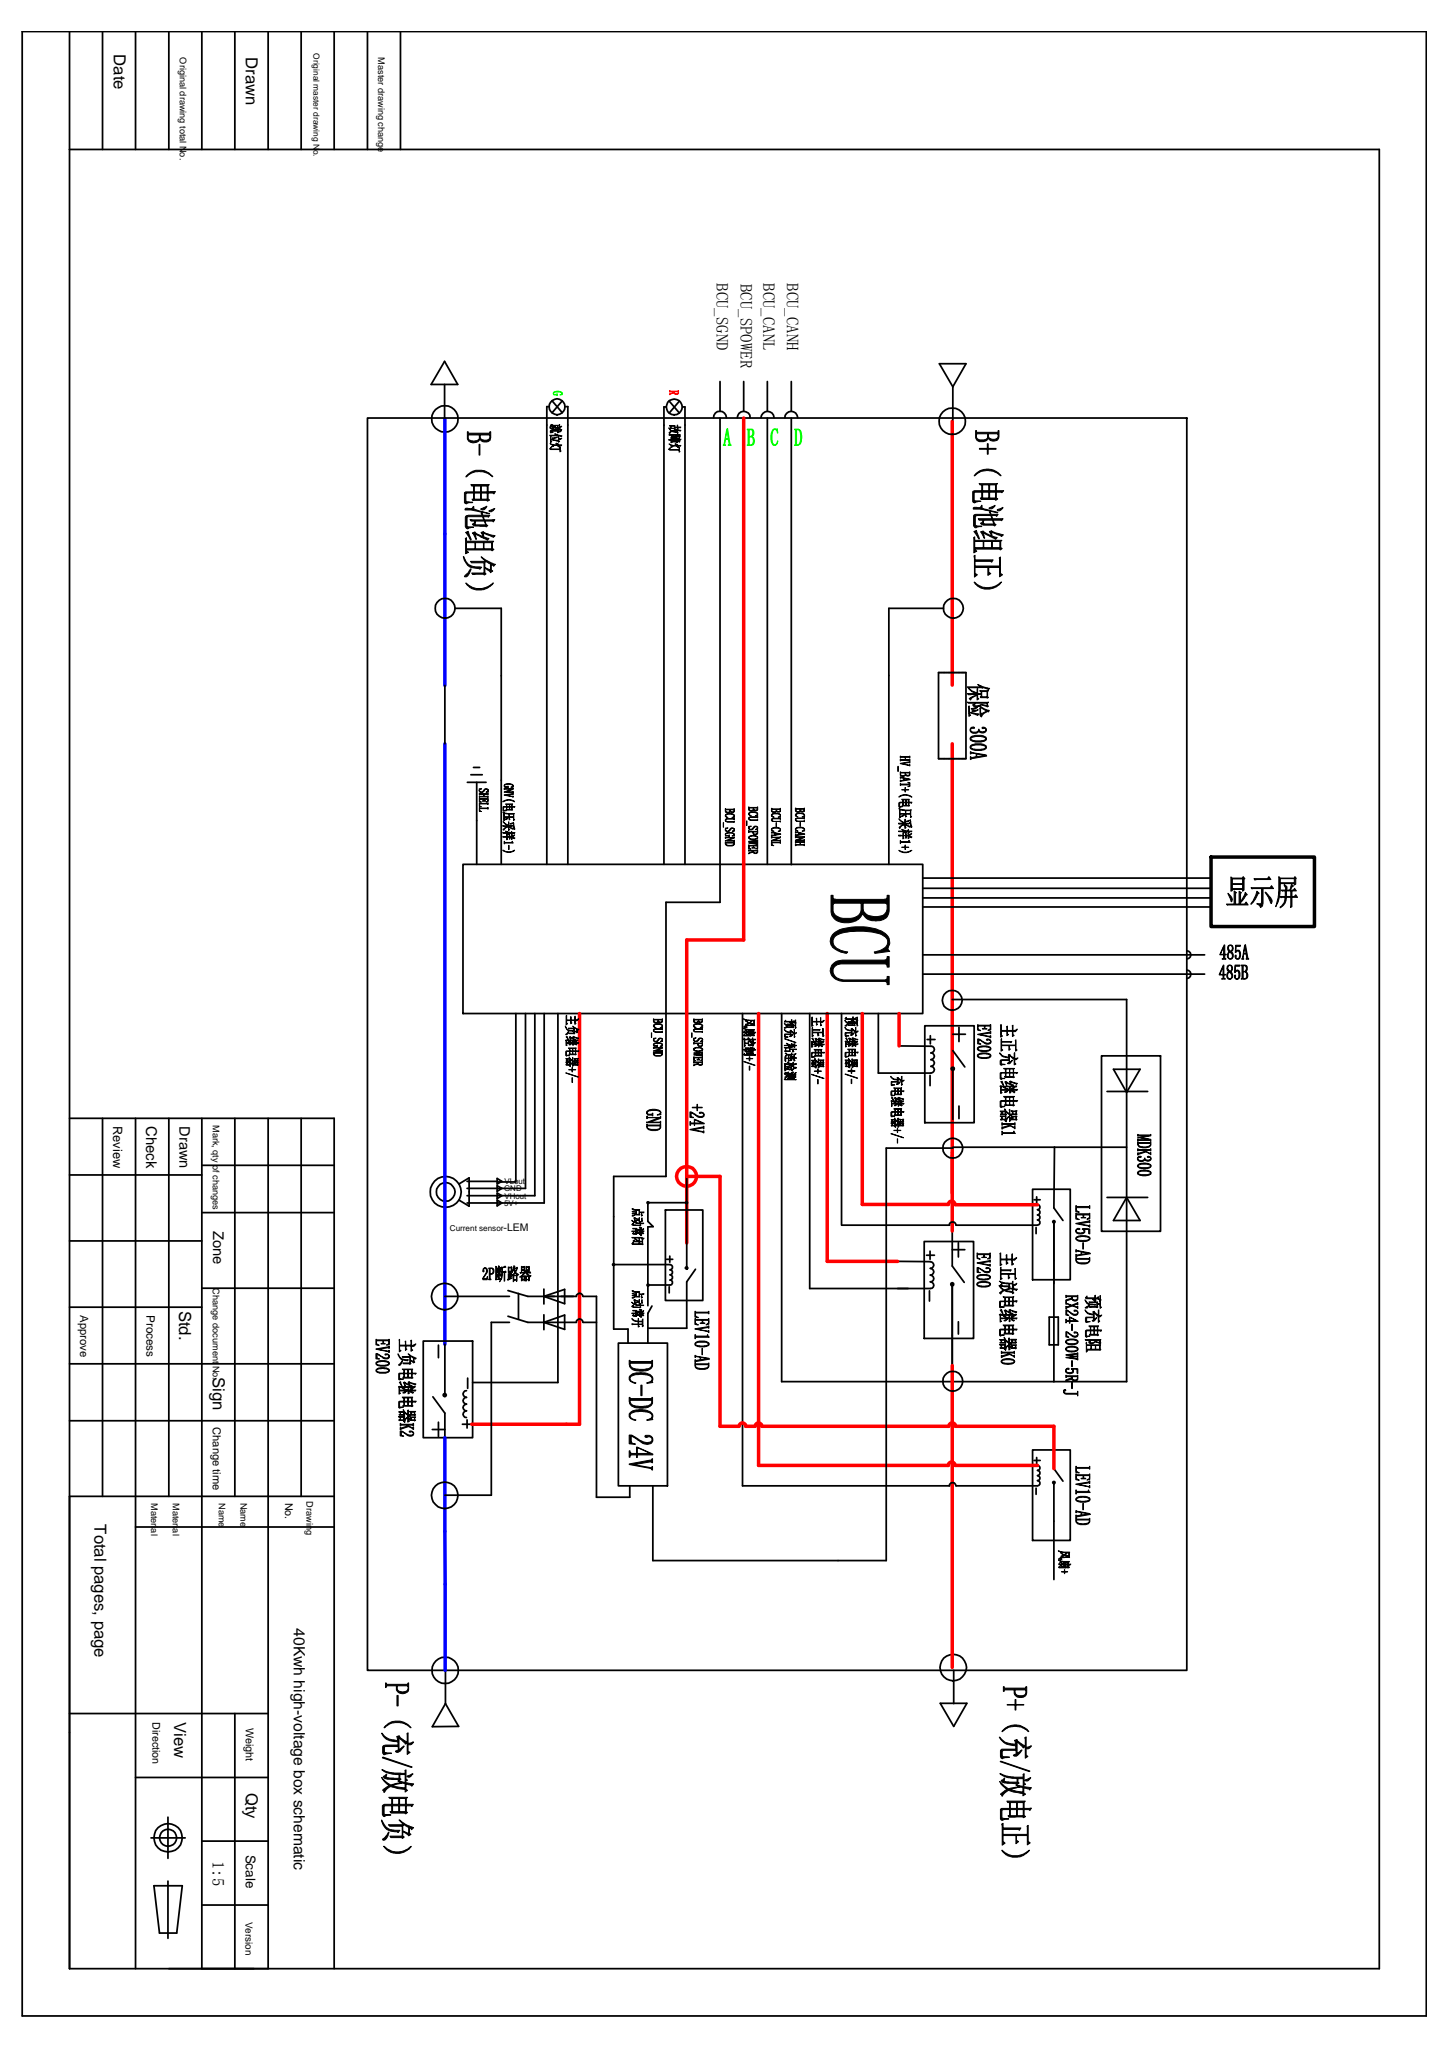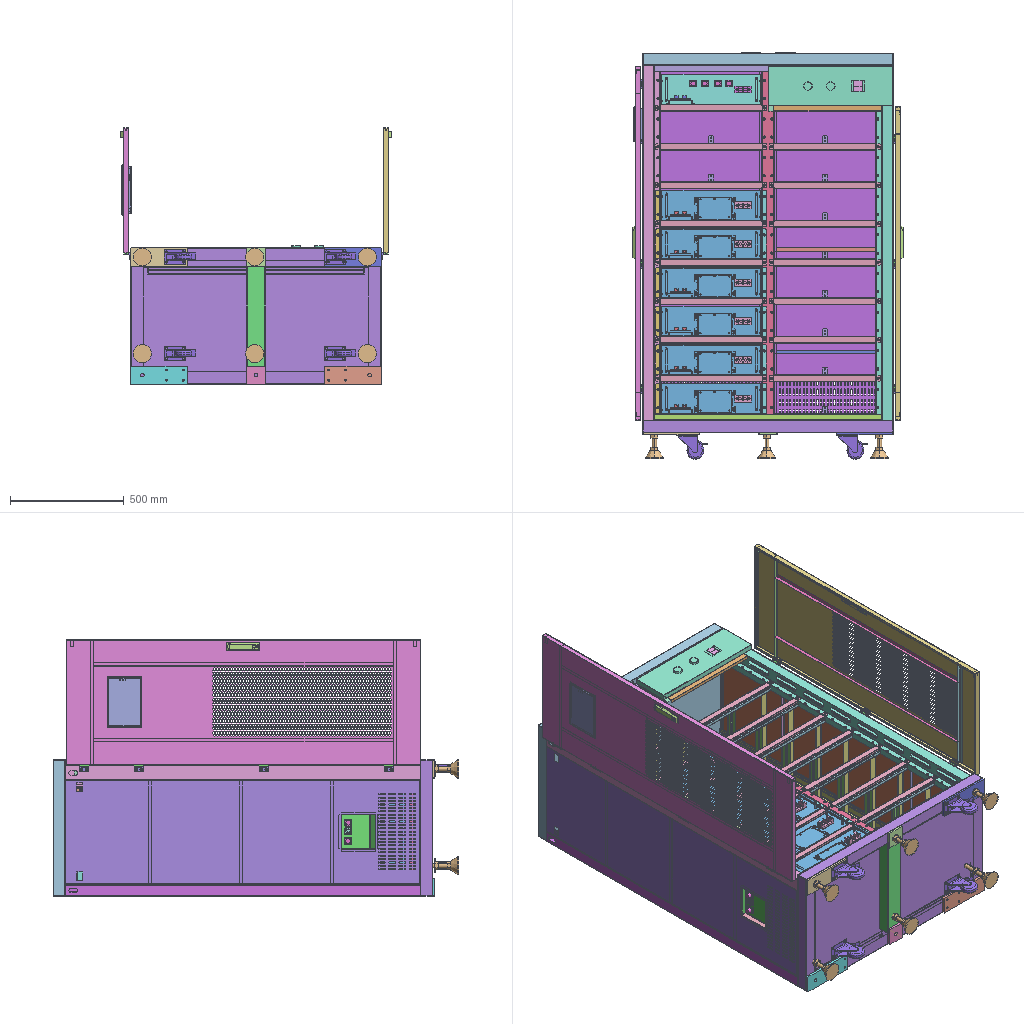Assembly | SolidWorks | 125 different items | 547 placed | box 1190 x 1786 x 1129 mm
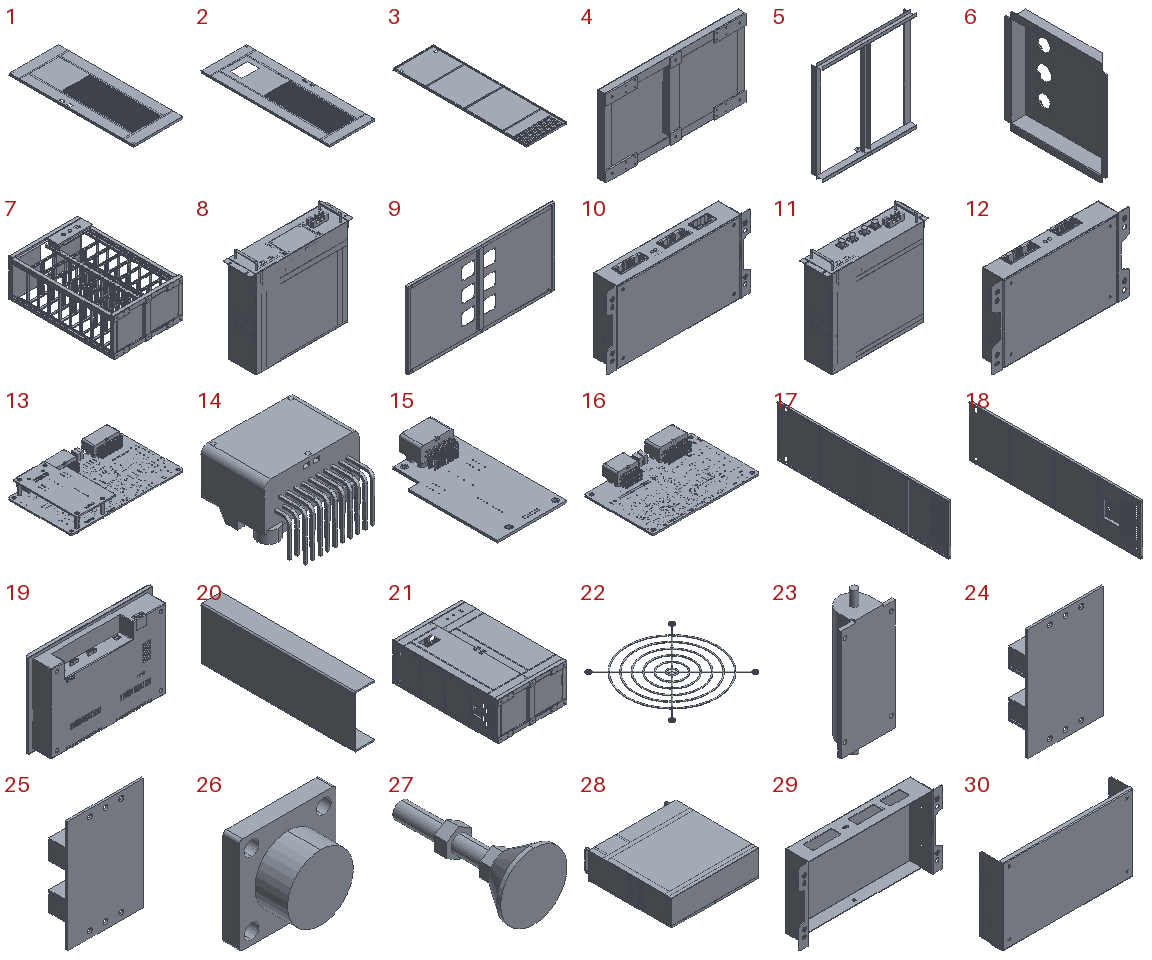Parts list (item | name | quantity | parent item | size | volume | features):
1 | (subassembly) | x1 | - | - | 1001235 mm3 | features MirrorCompFeat 1, ReferencePattern 1
2 | (subassembly) | x1 | - | - | 1107587 mm3 | features MirrorCompFeat 1, ReferencePattern 1
3 | (subassembly) | x2 | - | 473 x 1568 x 20 mm | 883759 mm3 | features CompositeCurve 2
4 | (subassembly) | x1 | in 7 | 1100 x 63 x 600.001 mm | 2743089 mm3 | -
5 | (subassembly) | x17 | in 7 | 453 x 63.5 x 481.5 mm | 236917 mm3 | -
6 | (subassembly) | x1 | in 18 | 29 x 171 x 172 mm | 45900 mm3 | -
7 | (subassembly) | x1 | - | - | 11157281 mm3 | features ReferencePattern 16, LocalLPattern 1
8 | (subassembly) | x6 | - | - | 10284410 mm3 | features ReferencePattern 16, CompositeCurve 5, LocalLPattern 2, MirrorCompFeat 1
9 | (subassembly) | x1 | - | 1035 x 20 x 535 mm | 656761 mm3 | -
10 | (subassembly) | x1 | in 11 | - | 121145 mm3 | -
11 | (subassembly) | x1 | - | - | 2990736 mm3 | features CompositeCurve 17, LocalLPattern 3, ReferencePattern 3
12 | (subassembly) | x6 | in 8 | 177.9 x 27.2 x 101.3 mm | 74977 mm3 | -
13 | (subassembly) | x1 | in 10 | - | 62246 mm3 | -
14 | (subassembly) | x1 | in 15 | 27.9 x 26.52 x 19.2 mm | 3570 mm3 | -
15 | (subassembly) | x1 | in 13 | 60 x 105.587 x 19.2 mm | 14940 mm3 | -
16 | (subassembly) | x6 | in 12 | 137.5 x 94.8 x 23.5 mm | 33178 mm3 | -
17 | (subassembly) | x1 | - | 20 x 1568 x 458 mm | 1656594 mm3 | features CompositeCurve 2
18 | (subassembly) | x1 | - | 30 x 1568 x 458 mm | 871583 mm3 | features CompositeCurve 3, LocalLPattern 1, ReferencePattern 1
19 | - | x1 | - | 227 x 40.02 x 153 mm | 206698 mm3 | features BaseBody 27
20 | - | x1 | in 7 | 23.5 x 176 x 60 mm | 27263 mm3 | features SplitBody 1
21 | - | x0 | - | - | 13322104 mm3 | features ICE 63, FlatPattern 34, SMBaseFlange 34, SheetMetal 34, LPattern 21, MirrorSolid 19, EdgeFlange 14, BossThin 9, MirrorPattern 6, SMMiteredFlange 6, Chamfer 2, CornerTrim 1, Split 1
22 | - | x6 | - | 89 x 89 x 1 mm | 913.094 mm3 | features Fillet 4, ICE 3, Extrusion 1, Revolution 1
23 | - | x1 | in 11 | 48 x 25.9 x 126 mm | 68546 mm3 | features ICE 7, Extrusion 1
24 | - | x6 | in 8 | 60.4 x 15.3 x 89.7 mm | 16280 mm3 | features ICE 4, Extrusion 1
25 | - | x1 | in 11 | 60.4 x 15.3 x 89.7 mm | 16562 mm3 | features ICE 3, Extrusion 1
26 | - | x1 | - | 29.5 x 17 x 29.5 mm | 7218 mm3 | features ICE 5, Extrusion 1, Fillet 1
27 | - | x6 | - | 80 x 160 x 80 mm | 165736 mm3 | features ICE 4, Extrusion 1
28 | - | x1 | in 11 | 437 x 449.5 x 132 mm | 767937 mm3 | features ICE 25, BossThin 16, LPattern 10, EdgeFlange 7, SMBaseFlange 7, FlatPattern 6, SheetMetal 6, MirrorPattern 4, CornerTrim 2, MirrorSolid 1, Split 1, Sweep 1
29 | - | x1 | in 10 | 216.4 x 35.2 x 109.5 mm | 30574 mm3 | features BaseBody 5
30 | - | x1 | in 10 | 185.4 x 34 x 108 mm | 28122 mm3 | features BaseBody 6
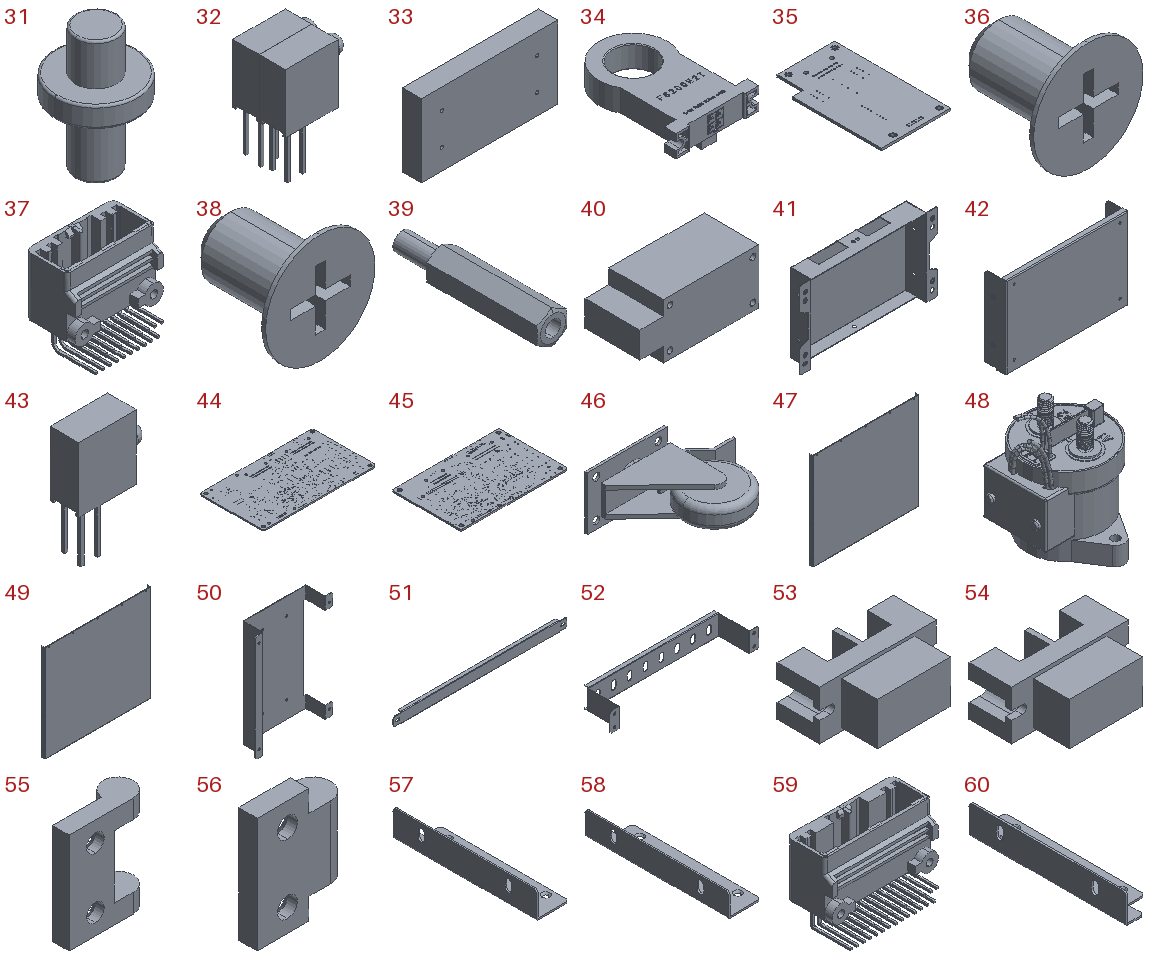31 | - | x8 | in 3, 17, 18 | 8 x 8 x 12 mm | 225.557 mm3 | features Fillet 2, ICE 2, Extrusion 1
32 | - | x1 | in 13 | 11.4 x 8.95 x 17.5 mm | 805.198 mm3 | features BaseBody 2
33 | - | x1 | in 11 | 215 x 30 x 115 mm | 739394 mm3 | features Extrusion 1, ICE 1
34 | - | x1 | in 11 | 56 x 80 x 24.3 mm | 37324 mm3 | features BaseBody 5
35 | - | x1 | in 15 | 60 x 100 x 2.001 mm | 11370 mm3 | features BaseBody 1
36 | - | x30 | in 12 | 5.5 x 5 x 5.5 mm | 40.626 mm3 | features BaseBody 1
37 | - | x6 | in 16 | 27.9 x 19.2 x 26.52 mm | 3570 mm3 | features BaseBody 1
38 | - | x5 | in 10 | 5.5 x 5 x 5.5 mm | 40.626 mm3 | features BaseBody 1
39 | - | x4 | in 13 | 4.7 x 24 x 5.427 mm | 364.722 mm3 | features BaseBody 1
40 | - | x1 | in 11 | 115 x 53 x 53 mm | 283866 mm3 | features ICE 2, Extrusion 1
41 | - | x6 | in 12 | 177.9 x 27.2 x 100 mm | 21775 mm3 | features BaseBody 5, ICE 2
42 | - | x6 | in 12 | 146.9 x 26 x 98.5 mm | 19821 mm3 | features BaseBody 6
43 | - | x12 | in 16 | 11.4 x 4.45 x 17.5 mm | 402.599 mm3 | features BaseBody 1
44 | - | x1 | in 13 | 177 x 100 x 2 mm | 34913 mm3 | features BaseBody 1
45 | - | x6 | in 16 | 137.5 x 89 x 2 mm | 24002 mm3 | features BaseBody 1
46 | - | x4 | - | 138.347 x 107 x 64 mm | 180748 mm3 | features ICE 7, BossThin 1, Extrusion 1, Fillet 1, MirrorPattern 1
47 | - | x6 | in 8 | 437.001 x 12.7 x 399 mm | 225419 mm3 | features ICE 3, LPattern 3, EdgeFlange 1, FlatPattern 1, SMBaseFlange 1, SheetMetal 1
48 | - | x3 | in 11 | - | - | features BaseBody 14, RefSurface 2
49 | - | x1 | in 11 | 437.001 x 12.7 x 399 mm | 225419 mm3 | features ICE 3, LPattern 3, EdgeFlange 1, FlatPattern 1, SMBaseFlange 1, SheetMetal 1
50 | - | x1 | in 11 | 160 x 41 x 220 mm | 42307 mm3 | features ICE 3, CornerTrim 1, FlatPattern 1, SMBaseFlange 1, SheetMetal 1
51 | - | x17 | - | 490 x 9.5 x 29 mm | 30933 mm3 | features CornerTrim 2, ICE 2, EdgeFlange 1, FlatPattern 1, SMBaseFlange 1, SheetMetal 1
52 | - | x12 | in 8 | 385 x 91.2 x 52.6 mm | 39000 mm3 | features CornerTrim 2, ICE 2, EdgeFlange 1, FlatPattern 1, LPattern 1, MirrorPattern 1, SMBaseFlange 1, SheetMetal 1
53 | - | x7 | in 8, 11 | 71 x 48 x 30 mm | 59444 mm3 | features ICE 5, LPattern 2, Extrusion 1
54 | - | x1 | in 11 | 71 x 48 x 30 mm | 59444 mm3 | features ICE 5, LPattern 2, Extrusion 1
55 | - | x7 | - | 31.5 x 12 x 40 mm | 5884 mm3 | features ICE 3, Chamfer 1, Extrusion 1
56 | - | x7 | - | 31.5 x 12 x 40 mm | 7190 mm3 | features ICE 3, Chamfer 1, Extrusion 1
57 | - | x6 | in 8 | 30 x 132 x 24.5 mm | 9772 mm3 | features ICE 3, CornerTrim 2, Chamfer 1, EdgeFlange 1, FlatPattern 1, SMBaseFlange 1, SheetMetal 1
58 | - | x1 | in 11 | 30 x 132 x 21.5 mm | 9178 mm3 | features ICE 3, CornerTrim 2, Chamfer 1, EdgeFlange 1, FlatPattern 1, SMBaseFlange 1, SheetMetal 1
59 | - | x6 | in 16 | 36.7 x 19.2 x 26.52 mm | 4801 mm3 | features BaseBody 1
60 | - | x6 | in 8 | 30 x 132 x 24.5 mm | 9772 mm3 | features ICE 3, CornerTrim 2, Chamfer 1, EdgeFlange 1, FlatPattern 1, SMBaseFlange 1, SheetMetal 1
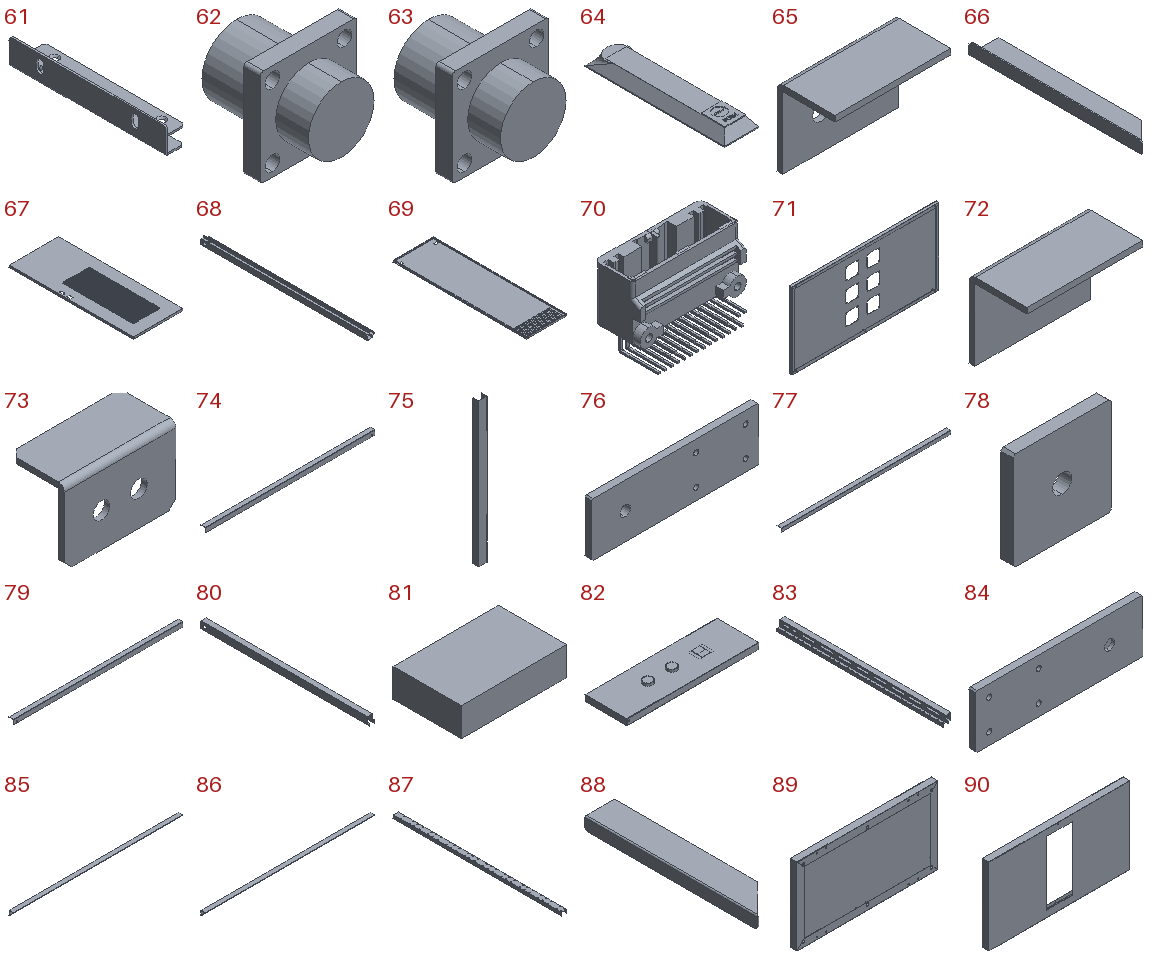61 | - | x1 | in 11 | 30 x 132 x 21.5 mm | 9178 mm3 | features ICE 3, CornerTrim 2, Chamfer 1, EdgeFlange 1, FlatPattern 1, SMBaseFlange 1, SheetMetal 1
62 | - | x2 | in 18 | 29.5 x 32 x 29.5 mm | 13059 mm3 | features ICE 3, Extrusion 1, Fillet 1
63 | - | x7 | in 11 | 29.5 x 32 x 29.5 mm | 13059 mm3 | features ICE 3, Extrusion 1, Fillet 1
64 | - | x2 | - | 36 x 147 x 22 mm | 47748 mm3 | features ICE 7, Blend 1
65 | - | x1 | in 1 | 30 x 15 x 20 mm | 1467 mm3 | features SplitBody 1
66 | - | x2 | in 6 | 26 x 152.414 x 11 mm | 5106 mm3 | features Chamfer 1, SplitBody 1
67 | - | x1 | in 1 | - | 901545 mm3 | features APattern 1, ICE 1, SplitBody 1
68 | - | x1 | in 7 | 75 x 1562 x 70 mm | 454767 mm3 | features SplitBody 1
69 | - | x2 | in 3 | 473 x 1560 x 20 mm | 829157 mm3 | features LPattern 2, ICE 1, SplitBody 1
70 | - | x1 | in 13 | 36.7 x 19.2 x 26.52 mm | 4801 mm3 | features BaseBody 1
71 | - | x1 | in 9 | 1035 x 20 x 535 mm | 624346 mm3 | features SplitBody 1
72 | - | x1 | in 2 | 30 x 15 x 20 mm | 1467 mm3 | features SplitBody 1
73 | - | x1 | in 1 | 30 x 15 x 20 mm | 1431 mm3 | features Chamfer 1, ICE 1, SplitBody 1
74 | - | x1 | in 2 | 547.1 x 15 x 15 mm | 15709 mm3 | features SplitBody 1
75 | - | x1 | in 9 | 30 x 19 x 495 mm | 32415 mm3 | features SplitBody 1
76 | - | x1 | in 4 | 250 x 10 x 80 mm | 196266 mm3 | features ICE 1, SplitBody 1
77 | - | x1 | in 7 | 1000 x 26.5 x 20 mm | 66953 mm3 | features SplitBody 1
78 | - | x1 | in 4 | 80 x 10 x 80 mm | 62033 mm3 | features SplitBody 1
79 | - | x1 | in 1 | 547.1 x 15 x 15 mm | 15709 mm3 | features SplitBody 1
80 | - | x1 | in 7 | 75 x 1562 x 90 mm | 569979 mm3 | features SplitBody 1
81 | - | x96 | in 8 | 148.9 x 100.6 x 40.2 mm | 574008 mm3 | features Extrusion 1, ICE 1
82 | - | x1 | in 7 | 548.5 x 174 x 73 mm | 187457 mm3 | features ICE 5, EdgeFlange 2, FlatPattern 2, SheetMetal 2, BossThin 1, CornerTrim 1, MirrorSolid 1, SMBaseFlange 1, SplitBody 1
83 | - | x1 | in 7 | 75 x 1562 x 90 mm | 568326 mm3 | features SplitBody 1
84 | - | x1 | in 4 | 250 x 10 x 80 mm | 198093 mm3 | features SplitBody 1
85 | - | x1 | in 2 | 547.1 x 15 x 15 mm | 15709 mm3 | features SplitBody 1
86 | - | x1 | in 1 | 547.1 x 15 x 15 mm | 15693 mm3 | features ICE 1, SplitBody 1
87 | - | x1 | in 7 | 50 x 1562 x 30 mm | 258598 mm3 | features SplitBody 1
88 | - | x1 | in 6 | 26 x 152.414 x 11 mm | 5106 mm3 | features Chamfer 1, SplitBody 1
89 | - | x1 | in 4 | 1100 x 53 x 600.001 mm | 1504531 mm3 | features SplitBody 1
90 | - | x1 | in 7 | 1100 x 53 x 600.001 mm | 1427839 mm3 | features SplitBody 1
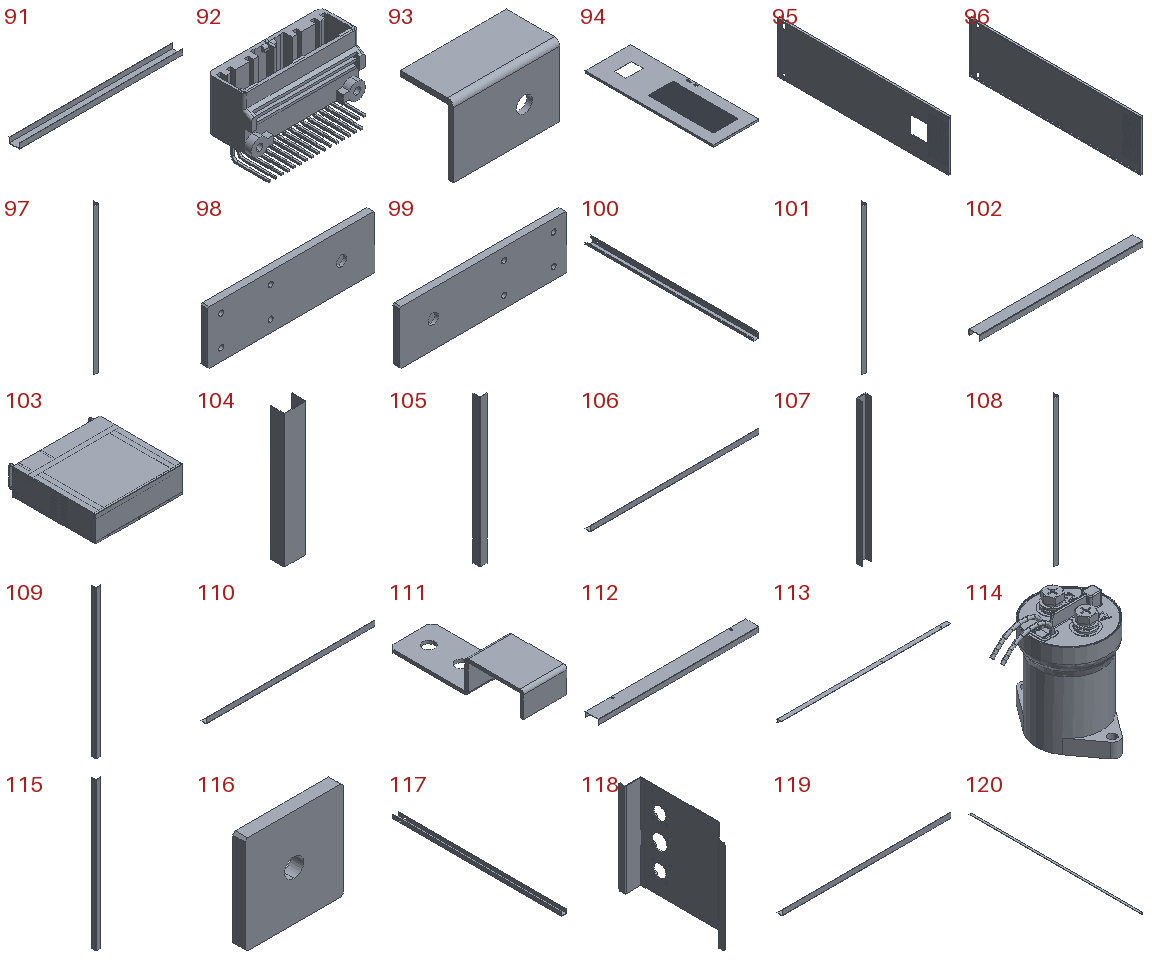91 | - | x17 | in 5 | 450 x 30 x 15 mm | 37982 mm3 | features SplitBody 1
92 | - | x1 | in 13 | 41.1 x 19.2 x 26.52 mm | 5328 mm3 | features BaseBody 1
93 | - | x1 | in 2 | 30 x 15 x 20 mm | 1467 mm3 | features SplitBody 1
94 | - | x1 | in 2 | - | 997556 mm3 | features APattern 1, ICE 1, SplitBody 1
95 | - | x1 | in 18 | 20 x 1560 x 458 mm | 785912 mm3 | features SplitBody 1
96 | - | x2 | in 17 | 20 x 1560 x 458 mm | 808412 mm3 | features SplitBody 1
97 | - | x1 | in 17 | 15 x 15 x 456 mm | 13107 mm3 | features SplitBody 1
98 | - | x1 | in 4 | 250 x 10 x 80 mm | 198093 mm3 | features SplitBody 1
99 | - | x1 | in 4 | 250 x 10 x 80 mm | 198093 mm3 | features SplitBody 1
100 | - | x1 | in 7 | 75 x 1562 x 70 mm | 454767 mm3 | features SplitBody 1
101 | - | x1 | in 17 | 15 x 15 x 456 mm | 13107 mm3 | features SplitBody 1
102 | - | x17 | in 5 | 450 x 30 x 15 mm | 37982 mm3 | features SplitBody 1
103 | - | x6 | in 8 | 437 x 449.5 x 132 mm | 626623 mm3 | features ICE 15, LPattern 7, SMBaseFlange 7, EdgeFlange 6, FlatPattern 6, SheetMetal 6, MirrorPattern 4, BossThin 3, CornerTrim 2, MirrorSolid 1, Split 1, Sweep 1
104 | - | x2 | in 4 | 80 x 51.5 x 487 mm | 130957 mm3 | features SplitBody 1
105 | - | x17 | in 5 | 21.5 x 21.5 x 450 mm | 27766 mm3 | features SplitBody 1
106 | - | x4 | in 3 | 471 x 15 x 15 mm | 13538 mm3 | features SplitBody 1
107 | - | x34 | in 5 | 30 x 20 x 450 mm | 44732 mm3 | features SplitBody 1
108 | - | x1 | in 17 | 15 x 15 x 456 mm | 13107 mm3 | features SplitBody 1
109 | - | x1 | in 18 | 15 x 15 x 456 mm | 13107 mm3 | features SplitBody 1
110 | - | x2 | in 3 | 471 x 15 x 15 mm | 13538 mm3 | features SplitBody 1
111 | - | x17 | in 5 | 20 x 62 x 15 mm | 2455 mm3 | features SplitBody 1
112 | - | x1 | in 7 | 475 x 40 x 15 mm | 32008 mm3 | features SplitBody 1
113 | - | x1 | in 7 | 1000 x 26.5 x 20 mm | 66881 mm3 | features SplitBody 1
114 | - | x1 | in 11 | - | - | features BaseBody 11, RefSurface 2
115 | - | x1 | in 18 | 15 x 15 x 456 mm | 13107 mm3 | features SplitBody 1
116 | - | x1 | in 4 | 80 x 10 x 80 mm | 62033 mm3 | features SplitBody 1
117 | - | x1 | in 7 | 50 x 1562 x 35 mm | 271759 mm3 | features SplitBody 1
118 | - | x1 | in 6 | 29 x 171 x 150 mm | 30583 mm3 | features ICE 5, BossThin 2, Chamfer 1, MirrorPattern 1, SplitBody 1
119 | - | x2 | in 3 | 471 x 15 x 15 mm | 13538 mm3 | features SplitBody 1
120 | - | x2 | in 1 | 15 x 1138 x 15 mm | 32695 mm3 | features SplitBody 1
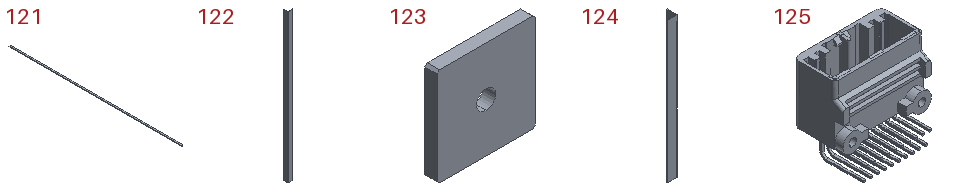121 | - | x2 | in 2 | 15 x 1317 x 15 mm | 37839 mm3 | features SplitBody 1
122 | - | x1 | in 18 | 15 x 15 x 456 mm | 13107 mm3 | features SplitBody 1
123 | - | x1 | in 4 | 80 x 10 x 80 mm | 62033 mm3 | features SplitBody 1
124 | - | x17 | in 5 | 31.5 x 31.5 x 450 mm | 41266 mm3 | features SplitBody 1
125 | - | x1 | in 14 | 27.9 x 19.2 x 26.52 mm | 3570 mm3 | features BaseBody 1
Mates (type | each side: item.copy, entity, surface, feature):
In the top assembly
DistanceDim | 67.1 face plane BasePart-Battery Cabinet-1 | 89.1 face plane BasePart-Battery Cabinet-1
DistanceDim | 89.1 face plane BasePart-Battery Cabinet-1 | 94.1 face plane BasePart-Battery Cabinet-1
Coincident | 83.1 face plane BasePart-Battery Cabinet-1 | 55.1 face plane Boss-Extrude 1
Concentric | 83.1 face cylinder BasePart-Battery Cabinet-1 | 55.1 face cylinder Cut-Extrude 2 | 2 times
Coincident | 80.1 face plane BasePart-Battery Cabinet-1 | 55.2 face plane Boss-Extrude 1
Concentric | 80.1 face cylinder BasePart-Battery Cabinet-1 | 55.2 edge
Concentric | 80.1 face cylinder BasePart-Battery Cabinet-1 | 55.2 face cylinder Cut-Extrude 2
Coincident | 94.1 face plane BasePart-Battery Cabinet-1 | 56.1 face plane Boss-Extrude 1
Concentric | 94.1 face cylinder BasePart-Battery Cabinet-1 | 56.1 edge | 2 times
Concentric | 67.1 face cylinder BasePart-Battery Cabinet-1 | 56.2 face cylinder Cut-Extrude 2 | 2 times
Concentric | 55.2 face cylinder Boss-Extrude 2 | 56.1 face cylinder Boss-Extrude 2
Concentric | 55.1 face cylinder Boss-Extrude 2 | 56.2 face cylinder Boss-Extrude 2
Coincident | 67.1 face plane BasePart-Battery Cabinet-1 | 56.2 face plane Boss-Extrude 1
Coincident | 80.1 face plane BasePart-Battery Cabinet-1 | 51.1 face plane Base-Flange 1
DistanceDim | 80.1 face cylinder BasePart-Battery Cabinet-1 | 51.1 face plane Cut-Extrude 2
Coincident | 94.1 face plane BasePart-Battery Cabinet-1 | 19.1 face plane Import 7
DistanceDim | 19.1 face plane Import 7 | 94.1 face plane BasePart-Battery Cabinet-1 | 2 times
Concentric | 94.1 face cylinder BasePart-Battery Cabinet-1 | 64.1 face cylinder Boss-Extrude 6 | 2 times
Coincident | 94.1 face plane BasePart-Battery Cabinet-1 | 64.1 face plane Boss-Extrude 2
Concentric | 67.1 face cylinder BasePart-Battery Cabinet-1 | 64.2 face cylinder Boss-Extrude 6 | 2 times
Coincident | 67.1 face plane BasePart-Battery Cabinet-1 | 64.2 face plane Boss-Extrude 2
Coincident | 118.1 face plane BasePart-Battery Cabinet-1 | 63.1 face plane Boss-Extrude 2
Concentric | 118.1 edge | 63.1 face cylinder Boss-Extrude 3
Coincident | 118.1 face plane BasePart-Battery Cabinet-1 | 26.1 face plane Boss-Extrude 2
Tangent | 26.1 face cylinder Boss-Extrude 1 | 118.1 face cylinder Cut-Extrude 3
Concentric | 99.1 face cylinder BasePart-Battery Cabinet-1 | 27.1 face cylinder Boss-Extrude 2
Coincident | 99.1 face plane BasePart-Battery Cabinet-1 | 27.1 face plane Boss-Extrude 5
Coincident | 99.1 face plane BasePart-Battery Cabinet-1 | 46.1 face plane Boss-Extrude 3
Concentric | 99.1 face cylinder BasePart-Battery Cabinet-1 | 46.1 face cylinder Cut-Extrude 1 | 2 times
Coincident | 71.1 face plane BasePart-Battery Cabinet-1 | 22.1 face plane Boss-Extrude 1
Concentric | 71.1 face cylinder BasePart-Battery Cabinet-1 | 22.1 face cylinder Cut-Extrude 1 | 2 times
Parallel | 91.1 face plane BasePart-Battery Cabinet-1 | 51.1 face plane Edge-Flange 1
DistanceDim | 51.1 face plane Edge-Flange 1 | 80.1 face plane BasePart-Battery Cabinet-1
Coincident | 91.1 face plane BasePart-Battery Cabinet-1 | 103.1 face plane Base-Flange 1
Coincident | 80.1 face plane BasePart-Battery Cabinet-1 | 60.1 face plane Edge-Flange 1
DistanceDim | 80.1 face plane BasePart-Battery Cabinet-1 | 60.1 face plane Base-Flange 1
Coincident | 105.1 face plane BasePart-Battery Cabinet-1 | 28.1 face plane Base-Flange 1
Coincident | assembly face | 28.1 face plane Edge-Flange 4 | 2 times
LimitPlanarAngleDim | 67.1 face plane BasePart-Battery Cabinet-1 | 90.1 face plane BasePart-Battery Cabinet-1
LimitPlanarAngleDim | 94.1 face plane BasePart-Battery Cabinet-1 | 113.1 face plane BasePart-Battery Cabinet-1
Coincident | 91.2 face plane BasePart-Battery Cabinet-1 | assembly face
In subassembly 3
Coincident | 69.1 face plane BasePart-Battery Cabinet-1 | 31.1 face plane Boss-Extrude 2
Concentric | 69.1 edge | 31.1 face cylinder Boss-Extrude 1
Coincident | 69.1 face plane BasePart-Battery Cabinet-1 | 31.2 face plane Boss-Extrude 2
Concentric | 69.1 edge | 31.2 face cylinder Boss-Extrude 1
In subassembly 8
Coincident | 103.2 face plane Base-Flange 1 | 8.1 plane
Coincident | 103.2 face plane Edge-Flange 4 | 47.1 face plane Edge-Flange 1 | 2 times
DistanceDim | 8.1 face | 103.2 face plane Edge-Flange 4
Coincident | 103.2 face plane Edge-Flange 4 | 57.1 face plane Base-Flange 1
Concentric | 103.2 face cylinder Cut-Extrude 1 | 57.1 edge | 2 times
Coincident | 103.2 face plane Edge-Flange 4 | 60.2 face plane Base-Flange 1
Concentric | 103.2 face cylinder Cut-Extrude 1 | 60.2 edge
Concentric | 103.2 face cylinder Cut-Extrude 7 | 53.1 face cylinder Cut-Extrude 2 | 2 times
Coincident | 103.2 face plane Edge-Flange 4 | 53.1 face plane Boss-Extrude 1
DistanceDim | 103.2 face plane Base-Flange 1 | 81.1 face plane Boss-Extrude 1
DistanceDim | 81.1 face plane Boss-Extrude 1 | 103.2 face plane Base-Flange 2
Coincident | 103.2 face plane Mirror 3 | 52.1 face plane Base-Flange 1
Concentric | 103.2 edge | 52.1 edge
Concentric | 103.2 face cylinder Cut-Extrude 8 | 52.1 face cylinder Cut-Extrude 1
DistanceDim | 103.2 face plane Edge-Flange 4 | 24.1 face plane Boss-Extrude 1
DistanceDim | 24.1 face plane Boss-Extrude 2 | 103.2 face plane Cut-Extrude 9 | 2 times
DistanceDim | 81.1 face plane Boss-Extrude 1 | 103.2 face plane Mirror 3
Coincident | 103.2 face plane Edge-Flange 4 | 42.1 face plane Import 4
Concentric | 103.2 face cylinder Boss-Extrude 2 | 41.1 face cylinder Cut-Extrude 2
Parallel | 103.2 face plane Edge-Flange 10 | 41.1 face plane Import 12
Coincident | 103.2 face plane Edge-Flange 8 | 47.1 face plane Base-Flange 1
In subassembly 18
Coincident | 95.1 face plane BasePart-Battery Cabinet-1 | 31.1 face plane Boss-Extrude 2
Concentric | 95.1 edge | 31.1 face cylinder Boss-Extrude 1
Coincident | 95.1 face plane BasePart-Battery Cabinet-1 | 31.2 face plane Boss-Extrude 2
Concentric | 95.1 face cylinder BasePart-Battery Cabinet-1 | 31.2 face cylinder Boss-Extrude 1
Coincident | 118.2 face plane BasePart-Battery Cabinet-1 | 62.1 face plane Boss-Extrude 2
Concentric | 118.2 edge | 62.1 edge
Concentric | 118.2 face cylinder Extrude-Thin 1 | 62.1 face cylinder Cut-Extrude 1
Coincident | 95.1 face plane BasePart-Battery Cabinet-1 | 66.1 face plane BasePart-Battery Cabinet-1
Coincident | 95.1 face plane BasePart-Battery Cabinet-1 | 118.2 face plane BasePart-Battery Cabinet-1 | 2 times
In subassembly 17
Coincident | 96.1 face plane BasePart-Battery Cabinet-1 | 31.1 face plane Boss-Extrude 2
Concentric | 96.1 edge | 31.1 face cylinder Boss-Extrude 1
Coincident | 31.1 face plane Boss-Extrude 2 | 31.2 face plane Boss-Extrude 2
Concentric | 96.2 edge | 31.2 face cylinder Boss-Extrude 1
In subassembly 11
Coincident | 28.2 face plane Base-Flange 1 | 11.1 plane
Coincident | 28.2 face plane Edge-Flange 4 | 49.1 face plane Edge-Flange 1 | 2 times
DistanceDim | 11.1 face | 28.2 face plane Edge-Flange 4
Coincident | 28.2 face plane Edge-Flange 4 | 58.1 face plane Base-Flange 1
Concentric | 28.2 face cylinder Cut-Extrude 1 | 58.1 edge | 2 times
Coincident | 28.2 face plane Edge-Flange 4 | 61.1 face plane Base-Flange 1
Concentric | 28.2 face cylinder Cut-Extrude 1 | 61.1 edge
Concentric | 28.2 face cylinder Cut-Extrude 7 | 54.1 face cylinder Cut-Extrude 2
Coincident | 28.2 face plane Edge-Flange 4 | 54.1 face plane Boss-Extrude 1
DistanceDim | 28.2 face plane Edge-Flange 4 | 25.1 face plane Boss-Extrude 1
DistanceDim | 25.1 face plane Boss-Extrude 2 | 28.2 face plane Cut-Extrude 9 | 2 times
Coincident | 28.2 face plane Edge-Flange 8 | 49.1 face plane Base-Flange 1
Coincident | 28.2 face plane Base-Flange 6 | 34.1 face plane Import 3
Concentric | 28.2 edge | 34.1 edge
Coincident | 28.2 face plane Edge-Flange 4 | 63.1 face plane Boss-Extrude 2
Concentric | 28.2 edge | 63.1 face cylinder Boss-Extrude 3
Parallel | 28.2 face plane Edge-Flange 8 | 63.1 face plane Boss-Extrude 2
Coincident | 28.2 face plane Base-Flange 6 | 23.1 face plane Boss-Extrude 1
Coincident | 28.2 face plane Base-Flange 6 | 50.1 face plane Base-Flange 1
Concentric | 28.2 face cylinder Cut-Extrude 27 | 50.1 face cylinder Cut-Extrude 2 | 2 times
Parallel | 28.2 face plane Edge-Flange 4 | 29.1 face plane Import 4
Coincident | 28.2 face plane Base-Flange 6 | 30.1 face plane Import 2
Coincident | 33.1 face plane Boss-Extrude 1 | 50.1 face plane Base-Flange 1
Concentric | 33.1 edge | 50.1 edge
Concentric | 33.1 face cylinder Cut-Extrude 1 | 50.1 edge
Parallel | 28.2 face plane Edge-Flange 4 | 23.1 face plane Boss-Extrude 1
Concentric | 28.2 edge | 23.1 edge | 2 times
Concentric | 28.2 edge | 40.1 face cylinder Cut-Extrude 2
Parallel | 28.2 face plane Edge-Flange 4 | 40.1 face plane Boss-Extrude 1
Coincident | 28.2 face plane Base-Flange 6 | 40.1 edge
Coincident | 63.1 face plane Boss-Extrude 2 | 63.2 face plane Boss-Extrude 2
Concentric | 28.2 edge | 63.2 edge
Coincident | 63.2 face plane Boss-Extrude 3 | 63.3 face plane Boss-Extrude 3
Concentric | 28.2 edge | 63.3 face cylinder Boss-Extrude 3
Coincident | 28.2 face plane Edge-Flange 4 | 53.1 face plane Boss-Extrude 1
Concentric | 28.2 face cylinder Extrude-Thin 2 | 53.1 face cylinder Cut-Extrude 2
Coincident | 28.2 face plane Base-Flange 6 | 48.1 face plane Import 12
Concentric | 28.2 face cylinder Extrude-Thin 13 | 48.1 face cylinder Import 12 | 2 times
Coincident | 28.2 face plane Base-Flange 6 | 48.2 face plane Import 12
Concentric | 28.2 face cylinder Extrude-Thin 8 | 48.2 face cylinder Import 12 | 2 times
Coincident | 28.2 face plane Base-Flange 6 | 114.1 face plane Import 9
Concentric | 28.2 face cylinder Extrude-Thin 15 | 114.1 face cylinder Import 9
Parallel | 28.2 face plane Edge-Flange 4 | 114.1 edge